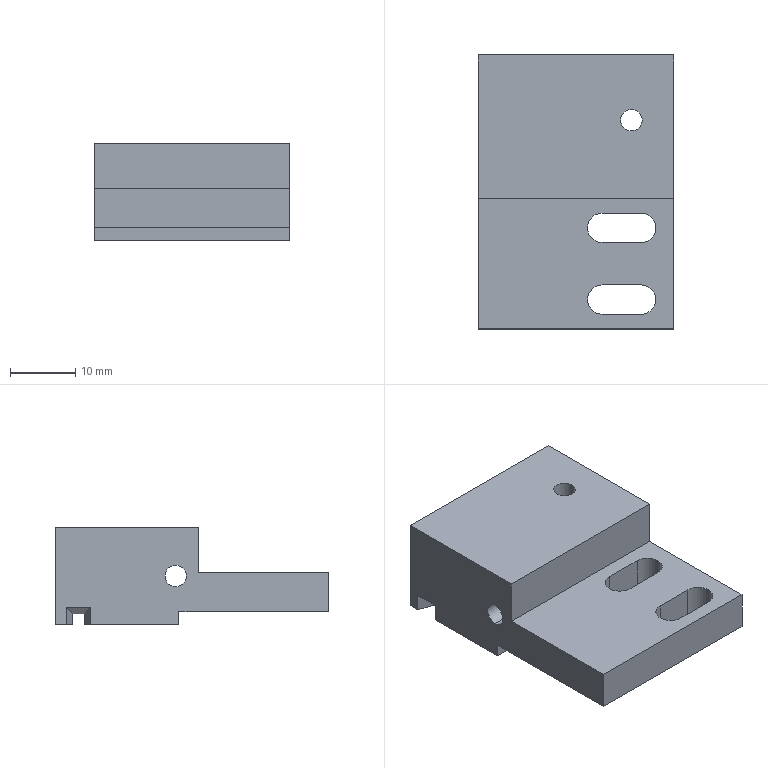Part | NX | features BREP 1 | 1 solid | 41 faces | box 30 x 42 x 15 mm | volume 11628 mm3 | plane 25 | cylinder 16 | commonest cylinder face diameters 4.5 x6 3.3 x4 10 x2 11.5 x2 14 x2
STEP:
#1=CARTESIAN_POINT('',(-23.5,-9.,-7.5));
#2=VERTEX_POINT('',#1);
#3=CARTESIAN_POINT('',(6.5,-9.,-7.5));
#4=VERTEX_POINT('',#3);
#5=CARTESIAN_POINT('',(6.5,-9.,-7.5));
#6=DIRECTION('',(1.,0.,0.));
#7=VECTOR('',#6,1000.);
#8=LINE('',#5,#7);
#9=EDGE_CURVE('',#2,#4,#8,.T.);
#10=ORIENTED_EDGE('',*,*,#9,.T.);
#11=CARTESIAN_POINT('',(6.5,-9.,-5.5));
#12=VERTEX_POINT('',#11);
#13=CARTESIAN_POINT('',(6.5,-9.,-5.5));
#14=DIRECTION('',(0.,0.,-1.));
#15=VECTOR('',#14,1000.);
#16=LINE('',#13,#15);
#17=EDGE_CURVE('',#12,#4,#16,.T.);
#18=ORIENTED_EDGE('',*,*,#17,.F.);
#19=CARTESIAN_POINT('',(-23.5,-9.,-5.5));
#20=VERTEX_POINT('',#19);
#21=CARTESIAN_POINT('',(6.5,-9.,-5.5));
#22=DIRECTION('',(1.,0.,0.));
#23=VECTOR('',#22,1000.);
#24=LINE('',#21,#23);
#25=EDGE_CURVE('',#20,#12,#24,.T.);
#26=ORIENTED_EDGE('',*,*,#25,.F.);
#27=CARTESIAN_POINT('',(-23.5,-9.,-5.5));
#28=DIRECTION('',(0.,0.,-1.));
#29=VECTOR('',#28,1000.);
#30=LINE('',#27,#29);
#31=EDGE_CURVE('',#20,#2,#30,.T.);
#32=ORIENTED_EDGE('',*,*,#31,.T.);
#33=EDGE_LOOP('',(#10,#18,#26,#32));
#34=FACE_BOUND('',#33,.T.);
#35=CARTESIAN_POINT('',(6.5,-9.,-5.5));
#36=DIRECTION('',(0.,1.,0.));
#37=DIRECTION('',(0.,0.,1.));
#38=AXIS2_PLACEMENT_3D('',#35,#36,#37);
#39=PLANE('',#38);
#40=ADVANCED_FACE('',(#34),#39,.F.);
#41=CARTESIAN_POINT('',(-4.5,-14.25,-5.5));
#42=VERTEX_POINT('',#41);
#43=CARTESIAN_POINT('',(-4.5,-18.75,-5.5));
#44=VERTEX_POINT('',#43);
#45=CARTESIAN_POINT('',(-4.5,-16.5,-5.5));
#46=DIRECTION('',(0.,0.,1.));
#47=DIRECTION('',(-1.,0.,0.));
#48=AXIS2_PLACEMENT_3D('',#45,#46,#47);
#49=CIRCLE('',#48,2.25);
#50=EDGE_CURVE('',#42,#44,#49,.T.);
#51=ORIENTED_EDGE('',*,*,#50,.T.);
#52=CARTESIAN_POINT('',(1.5,-18.75,-5.5));
#53=VERTEX_POINT('',#52);
#54=CARTESIAN_POINT('',(-4.5,-18.75,-5.5));
#55=DIRECTION('',(1.,0.,0.));
#56=VECTOR('',#55,1000.);
#57=LINE('',#54,#56);
#58=EDGE_CURVE('',#44,#53,#57,.T.);
#59=ORIENTED_EDGE('',*,*,#58,.T.);
#60=CARTESIAN_POINT('',(3.75,-16.5,-5.5));
#61=VERTEX_POINT('',#60);
#62=CARTESIAN_POINT('',(1.5,-16.5,-5.5));
#63=DIRECTION('',(0.,0.,1.));
#64=DIRECTION('',(-1.,0.,0.));
#65=AXIS2_PLACEMENT_3D('',#62,#63,#64);
#66=CIRCLE('',#65,2.25);
#67=EDGE_CURVE('',#53,#61,#66,.T.);
#68=ORIENTED_EDGE('',*,*,#67,.T.);
#69=CARTESIAN_POINT('',(1.5,-14.25,-5.5));
#70=VERTEX_POINT('',#69);
#71=CARTESIAN_POINT('',(1.5,-16.5,-5.5));
#72=DIRECTION('',(0.,0.,1.));
#73=DIRECTION('',(-1.,0.,0.));
#74=AXIS2_PLACEMENT_3D('',#71,#72,#73);
#75=CIRCLE('',#74,2.25);
#76=EDGE_CURVE('',#61,#70,#75,.T.);
#77=ORIENTED_EDGE('',*,*,#76,.T.);
#78=CARTESIAN_POINT('',(-4.5,-14.25,-5.5));
#79=DIRECTION('',(-1.,0.,0.));
#80=VECTOR('',#79,1000.);
#81=LINE('',#78,#80);
#82=EDGE_CURVE('',#70,#42,#81,.T.);
#83=ORIENTED_EDGE('',*,*,#82,.T.);
#84=EDGE_LOOP('',(#51,#59,#68,#77,#83));
#85=FACE_BOUND('',#84,.T.);
#86=CARTESIAN_POINT('',(-23.5,-32.,-5.5));
#87=VERTEX_POINT('',#86);
#88=CARTESIAN_POINT('',(-23.5,-9.,-5.5));
#89=DIRECTION('',(0.,1.,0.));
#90=VECTOR('',#89,1000.);
#91=LINE('',#88,#90);
#92=EDGE_CURVE('',#87,#20,#91,.T.);
#93=ORIENTED_EDGE('',*,*,#92,.T.);
#94=ORIENTED_EDGE('',*,*,#25,.T.);
#95=CARTESIAN_POINT('',(6.5,-32.,-5.5));
#96=VERTEX_POINT('',#95);
#97=CARTESIAN_POINT('',(6.5,-9.,-5.5));
#98=DIRECTION('',(0.,-1.,0.));
#99=VECTOR('',#98,1000.);
#100=LINE('',#97,#99);
#101=EDGE_CURVE('',#12,#96,#100,.T.);
#102=ORIENTED_EDGE('',*,*,#101,.T.);
#103=CARTESIAN_POINT('',(6.5,-32.,-5.5));
#104=DIRECTION('',(-1.,0.,0.));
#105=VECTOR('',#104,1000.);
#106=LINE('',#103,#105);
#107=EDGE_CURVE('',#96,#87,#106,.T.);
#108=ORIENTED_EDGE('',*,*,#107,.T.);
#109=EDGE_LOOP('',(#93,#94,#102,#108));
#110=FACE_BOUND('',#109,.T.);
#111=CARTESIAN_POINT('',(-4.5,-25.25,-5.5));
#112=VERTEX_POINT('',#111);
#113=CARTESIAN_POINT('',(-4.5,-29.75,-5.5));
#114=VERTEX_POINT('',#113);
#115=CARTESIAN_POINT('',(-4.5,-27.5,-5.5));
#116=DIRECTION('',(0.,0.,1.));
#117=DIRECTION('',(-1.,0.,0.));
#118=AXIS2_PLACEMENT_3D('',#115,#116,#117);
#119=CIRCLE('',#118,2.25);
#120=EDGE_CURVE('',#112,#114,#119,.T.);
#121=ORIENTED_EDGE('',*,*,#120,.T.);
#122=CARTESIAN_POINT('',(1.5,-29.75,-5.5));
#123=VERTEX_POINT('',#122);
#124=CARTESIAN_POINT('',(-4.5,-29.75,-5.5));
#125=DIRECTION('',(1.,0.,0.));
#126=VECTOR('',#125,1000.);
#127=LINE('',#124,#126);
#128=EDGE_CURVE('',#114,#123,#127,.T.);
#129=ORIENTED_EDGE('',*,*,#128,.T.);
#130=CARTESIAN_POINT('',(3.75,-27.5,-5.5));
#131=VERTEX_POINT('',#130);
#132=CARTESIAN_POINT('',(1.5,-27.5,-5.5));
#133=DIRECTION('',(0.,0.,1.));
#134=DIRECTION('',(-1.,0.,0.));
#135=AXIS2_PLACEMENT_3D('',#132,#133,#134);
#136=CIRCLE('',#135,2.25);
#137=EDGE_CURVE('',#123,#131,#136,.T.);
#138=ORIENTED_EDGE('',*,*,#137,.T.);
#139=CARTESIAN_POINT('',(1.5,-25.25,-5.5));
#140=VERTEX_POINT('',#139);
#141=CARTESIAN_POINT('',(1.5,-27.5,-5.5));
#142=DIRECTION('',(0.,0.,1.));
#143=DIRECTION('',(-1.,0.,0.));
#144=AXIS2_PLACEMENT_3D('',#141,#142,#143);
#145=CIRCLE('',#144,2.25);
#146=EDGE_CURVE('',#131,#140,#145,.T.);
#147=ORIENTED_EDGE('',*,*,#146,.T.);
#148=CARTESIAN_POINT('',(-4.5,-25.25,-5.5));
#149=DIRECTION('',(-1.,0.,0.));
#150=VECTOR('',#149,1000.);
#151=LINE('',#148,#150);
#152=EDGE_CURVE('',#140,#112,#151,.T.);
#153=ORIENTED_EDGE('',*,*,#152,.T.);
#154=EDGE_LOOP('',(#121,#129,#138,#147,#153));
#155=FACE_BOUND('',#154,.T.);
#156=CARTESIAN_POINT('',(0.,0.,-5.5));
#157=DIRECTION('',(0.,0.,-1.));
#158=DIRECTION('',(-1.,0.,0.));
#159=AXIS2_PLACEMENT_3D('',#156,#157,#158);
#160=PLANE('',#159);
#161=ADVANCED_FACE('',(#85,#110,#155),#160,.T.);
#162=CARTESIAN_POINT('',(-5.75,0.,-4.3));
#163=VERTEX_POINT('',#162);
#164=CARTESIAN_POINT('',(5.75,0.,-4.3));
#165=VERTEX_POINT('',#164);
#166=CARTESIAN_POINT('',(0.,0.,-4.3));
#167=DIRECTION('',(0.,0.,-1.));
#168=DIRECTION('',(-1.,0.,0.));
#169=AXIS2_PLACEMENT_3D('',#166,#167,#168);
#170=CIRCLE('',#169,5.75);
#171=EDGE_CURVE('',#163,#165,#170,.T.);
#172=ORIENTED_EDGE('',*,*,#171,.T.);
#173=CARTESIAN_POINT('',(0.,0.,-4.3));
#174=DIRECTION('',(0.,0.,-1.));
#175=DIRECTION('',(-1.,0.,0.));
#176=AXIS2_PLACEMENT_3D('',#173,#174,#175);
#177=CIRCLE('',#176,5.75);
#178=EDGE_CURVE('',#165,#163,#177,.T.);
#179=ORIENTED_EDGE('',*,*,#178,.T.);
#180=EDGE_LOOP('',(#172,#179));
#181=FACE_BOUND('',#180,.T.);
#182=CARTESIAN_POINT('',(-5.,0.,-4.3));
#183=VERTEX_POINT('',#182);
#184=CARTESIAN_POINT('',(5.,0.,-4.3));
#185=VERTEX_POINT('',#184);
#186=CARTESIAN_POINT('',(0.,0.,-4.3));
#187=DIRECTION('',(0.,0.,-1.));
#188=DIRECTION('',(-1.,0.,0.));
#189=AXIS2_PLACEMENT_3D('',#186,#187,#188);
#190=CIRCLE('',#189,5.);
#191=EDGE_CURVE('',#183,#185,#190,.T.);
#192=ORIENTED_EDGE('',*,*,#191,.F.);
#193=CARTESIAN_POINT('',(0.,0.,-4.3));
#194=DIRECTION('',(0.,0.,-1.));
#195=DIRECTION('',(-1.,0.,0.));
#196=AXIS2_PLACEMENT_3D('',#193,#194,#195);
#197=CIRCLE('',#196,5.);
#198=EDGE_CURVE('',#185,#183,#197,.T.);
#199=ORIENTED_EDGE('',*,*,#198,.F.);
#200=EDGE_LOOP('',(#192,#199));
#201=FACE_BOUND('',#200,.T.);
#202=CARTESIAN_POINT('',(0.,0.,-4.3));
#203=DIRECTION('',(0.,0.,-1.));
#204=DIRECTION('',(-1.,0.,0.));
#205=AXIS2_PLACEMENT_3D('',#202,#203,#204);
#206=PLANE('',#205);
#207=ADVANCED_FACE('',(#181,#201),#206,.T.);
#208=CARTESIAN_POINT('',(5.75,0.,-5.8));
#209=VERTEX_POINT('',#208);
#210=CARTESIAN_POINT('',(5.75,0.,-4.3));
#211=DIRECTION('',(0.,0.,-1.));
#212=VECTOR('',#211,1000.);
#213=LINE('',#210,#212);
#214=EDGE_CURVE('',#165,#209,#213,.T.);
#215=ORIENTED_EDGE('',*,*,#214,.F.);
#216=ORIENTED_EDGE('',*,*,#171,.F.);
#217=CARTESIAN_POINT('',(-5.75,0.,-5.8));
#218=VERTEX_POINT('',#217);
#219=CARTESIAN_POINT('',(-5.75,0.,-4.3));
#220=DIRECTION('',(0.,0.,-1.));
#221=VECTOR('',#220,1000.);
#222=LINE('',#219,#221);
#223=EDGE_CURVE('',#163,#218,#222,.T.);
#224=ORIENTED_EDGE('',*,*,#223,.T.);
#225=CARTESIAN_POINT('',(0.,0.,-5.8));
#226=DIRECTION('',(0.,0.,-1.));
#227=DIRECTION('',(-1.,0.,0.));
#228=AXIS2_PLACEMENT_3D('',#225,#226,#227);
#229=CIRCLE('',#228,5.75);
#230=EDGE_CURVE('',#218,#209,#229,.T.);
#231=ORIENTED_EDGE('',*,*,#230,.T.);
#232=EDGE_LOOP('',(#215,#216,#224,#231));
#233=FACE_BOUND('',#232,.T.);
#234=CARTESIAN_POINT('',(0.,0.,-4.3));
#235=DIRECTION('',(0.,0.,-1.));
#236=DIRECTION('',(-1.,0.,0.));
#237=AXIS2_PLACEMENT_3D('',#234,#235,#236);
#238=CYLINDRICAL_SURFACE('',#237,5.75);
#239=ADVANCED_FACE('',(#233),#238,.F.);
#240=CARTESIAN_POINT('',(-23.5,-8.5,-1.65));
#241=VERTEX_POINT('',#240);
#242=CARTESIAN_POINT('',(6.5,-8.5,-1.65));
#243=VERTEX_POINT('',#242);
#244=CARTESIAN_POINT('',(-23.5,-8.5,-1.65));
#245=DIRECTION('',(-1.,0.,0.));
#246=VECTOR('',#245,1000.);
#247=LINE('',#244,#246);
#248=EDGE_CURVE('',#241,#243,#247,.F.);
#249=ORIENTED_EDGE('',*,*,#248,.T.);
#250=CARTESIAN_POINT('',(6.5,-8.5,1.65));
#251=VERTEX_POINT('',#250);
#252=CARTESIAN_POINT('',(6.5,-8.5,0.));
#253=DIRECTION('',(-1.,0.,0.));
#254=DIRECTION('',(0.,0.,1.));
#255=AXIS2_PLACEMENT_3D('',#252,#253,#254);
#256=CIRCLE('',#255,1.65);
#257=EDGE_CURVE('',#251,#243,#256,.T.);
#258=ORIENTED_EDGE('',*,*,#257,.F.);
#259=CARTESIAN_POINT('',(-23.5,-8.5,1.65));
#260=VERTEX_POINT('',#259);
#261=CARTESIAN_POINT('',(-23.5,-8.5,1.65));
#262=DIRECTION('',(-1.,0.,0.));
#263=VECTOR('',#262,1000.);
#264=LINE('',#261,#263);
#265=EDGE_CURVE('',#260,#251,#264,.F.);
#266=ORIENTED_EDGE('',*,*,#265,.F.);
#267=CARTESIAN_POINT('',(-23.5,-8.5,0.));
#268=DIRECTION('',(-1.,0.,0.));
#269=DIRECTION('',(0.,0.,1.));
#270=AXIS2_PLACEMENT_3D('',#267,#268,#269);
#271=CIRCLE('',#270,1.65);
#272=EDGE_CURVE('',#260,#241,#271,.T.);
#273=ORIENTED_EDGE('',*,*,#272,.T.);
#274=EDGE_LOOP('',(#249,#258,#266,#273));
#275=FACE_BOUND('',#274,.T.);
#276=CARTESIAN_POINT('',(-23.5,-8.5,0.));
#277=DIRECTION('',(-1.,0.,0.));
#278=DIRECTION('',(0.,0.,1.));
#279=AXIS2_PLACEMENT_3D('',#276,#277,#278);
#280=CYLINDRICAL_SURFACE('',#279,1.65);
#281=ADVANCED_FACE('',(#275),#280,.F.);
#282=CARTESIAN_POINT('',(-4.899,5.5,-5.8));
#283=VERTEX_POINT('',#282);
#284=CARTESIAN_POINT('',(-4.899,5.,-5.8));
#285=VERTEX_POINT('',#284);
#286=CARTESIAN_POINT('',(-4.899,5.5,-5.8));
#287=DIRECTION('',(0.,-1.,0.));
#288=VECTOR('',#287,1000.);
#289=LINE('',#286,#288);
#290=EDGE_CURVE('',#283,#285,#289,.T.);
#291=ORIENTED_EDGE('',*,*,#290,.T.);
#292=CARTESIAN_POINT('',(-4.899,5.,-7.5));
#293=VERTEX_POINT('',#292);
#294=CARTESIAN_POINT('',(-4.899,5.,-5.043));
#295=DIRECTION('',(0.,0.,-1.));
#296=VECTOR('',#295,1000.);
#297=LINE('',#294,#296);
#298=EDGE_CURVE('',#285,#293,#297,.T.);
#299=ORIENTED_EDGE('',*,*,#298,.T.);
#300=CARTESIAN_POINT('',(-4.899,5.5,-7.5));
#301=VERTEX_POINT('',#300);
#302=CARTESIAN_POINT('',(-4.899,5.5,-7.5));
#303=DIRECTION('',(0.,-1.,0.));
#304=VECTOR('',#303,1000.);
#305=LINE('',#302,#304);
#306=EDGE_CURVE('',#301,#293,#305,.T.);
#307=ORIENTED_EDGE('',*,*,#306,.F.);
#308=CARTESIAN_POINT('',(-4.899,5.5,-5.043));
#309=DIRECTION('',(0.,0.,-1.));
#310=VECTOR('',#309,1000.);
#311=LINE('',#308,#310);
#312=EDGE_CURVE('',#283,#301,#311,.T.);
#313=ORIENTED_EDGE('',*,*,#312,.F.);
#314=EDGE_LOOP('',(#291,#299,#307,#313));
#315=FACE_BOUND('',#314,.T.);
#316=CARTESIAN_POINT('',(-4.899,5.5,-5.043));
#317=DIRECTION('',(1.,0.,0.));
#318=DIRECTION('',(0.,0.,-1.));
#319=AXIS2_PLACEMENT_3D('',#316,#317,#318);
#320=PLANE('',#319);
#321=ADVANCED_FACE('',(#315),#320,.T.);
#322=CARTESIAN_POINT('',(-23.5,4.5,-4.8));
#323=VERTEX_POINT('',#322);
#324=CARTESIAN_POINT('',(-20.5,5.5,-5.8));
#325=VERTEX_POINT('',#324);
#326=CARTESIAN_POINT('',(-26.855,3.382,-3.682));
#327=DIRECTION('',(0.9045,0.3015,-0.3015));
#328=VECTOR('',#327,1000.);
#329=LINE('',#326,#328);
#330=EDGE_CURVE('',#323,#325,#329,.T.);
#331=ORIENTED_EDGE('',*,*,#330,.T.);
#332=CARTESIAN_POINT('',(-20.5,5.5,-7.5));
#333=VERTEX_POINT('',#332);
#334=CARTESIAN_POINT('',(-20.5,5.5,-5.8));
#335=DIRECTION('',(0.,0.,1.));
#336=VECTOR('',#335,1000.);
#337=LINE('',#334,#336);
#338=EDGE_CURVE('',#333,#325,#337,.T.);
#339=ORIENTED_EDGE('',*,*,#338,.F.);
#340=CARTESIAN_POINT('',(-23.5,4.5,-7.5));
#341=VERTEX_POINT('',#340);
#342=CARTESIAN_POINT('',(-3.7,11.1,-7.5));
#343=DIRECTION('',(0.9487,0.3162,0.));
#344=VECTOR('',#343,1000.);
#345=LINE('',#342,#344);
#346=EDGE_CURVE('',#341,#333,#345,.T.);
#347=ORIENTED_EDGE('',*,*,#346,.F.);
#348=CARTESIAN_POINT('',(-23.5,4.5,-7.5));
#349=DIRECTION('',(0.,0.,-1.));
#350=VECTOR('',#349,1000.);
#351=LINE('',#348,#350);
#352=EDGE_CURVE('',#323,#341,#351,.T.);
#353=ORIENTED_EDGE('',*,*,#352,.F.);
#354=EDGE_LOOP('',(#331,#339,#347,#353));
#355=FACE_BOUND('',#354,.T.);
#356=CARTESIAN_POINT('',(-23.5,4.5,7.5));
#357=DIRECTION('',(-0.3162,0.9487,0.));
#358=DIRECTION('',(0.,0.,1.));
#359=AXIS2_PLACEMENT_3D('',#356,#357,#358);
#360=PLANE('',#359);
#361=ADVANCED_FACE('',(#355),#360,.T.);
#362=CARTESIAN_POINT('',(-23.5,8.3,-4.8));
#363=VERTEX_POINT('',#362);
#364=CARTESIAN_POINT('',(-20.5,7.3,-5.8));
#365=VERTEX_POINT('',#364);
#366=CARTESIAN_POINT('',(-12.509,4.636,-8.464));
#367=DIRECTION('',(0.9045,-0.3015,-0.3015));
#368=VECTOR('',#367,1000.);
#369=LINE('',#366,#368);
#370=EDGE_CURVE('',#363,#365,#369,.T.);
#371=ORIENTED_EDGE('',*,*,#370,.T.);
#372=CARTESIAN_POINT('',(-20.5,0.,-5.8));
#373=DIRECTION('',(0.,1.,0.));
#374=VECTOR('',#373,1000.);
#375=LINE('',#372,#374);
#376=EDGE_CURVE('',#325,#365,#375,.T.);
#377=ORIENTED_EDGE('',*,*,#376,.F.);
#378=ORIENTED_EDGE('',*,*,#330,.F.);
#379=CARTESIAN_POINT('',(-23.5,-32.,-4.8));
#380=DIRECTION('',(0.,-1.,0.));
#381=VECTOR('',#380,1000.);
#382=LINE('',#379,#381);
#383=EDGE_CURVE('',#363,#323,#382,.T.);
#384=ORIENTED_EDGE('',*,*,#383,.F.);
#385=EDGE_LOOP('',(#371,#377,#378,#384));
#386=FACE_BOUND('',#385,.T.);
#387=CARTESIAN_POINT('',(-23.5,-32.,-4.8));
#388=DIRECTION('',(0.3162,0.,0.9487));
#389=DIRECTION('',(0.,-1.,0.));
#390=AXIS2_PLACEMENT_3D('',#387,#388,#389);
#391=PLANE('',#390);
#392=ADVANCED_FACE('',(#386),#391,.F.);
#393=CARTESIAN_POINT('',(-20.5,7.3,-7.5));
#394=VERTEX_POINT('',#393);
#395=CARTESIAN_POINT('',(-23.5,8.3,-7.5));
#396=VERTEX_POINT('',#395);
#397=CARTESIAN_POINT('',(0.14,0.42,-7.5));
#398=DIRECTION('',(-0.9487,0.3162,0.));
#399=VECTOR('',#398,1000.);
#400=LINE('',#397,#399);
#401=EDGE_CURVE('',#394,#396,#400,.T.);
#402=ORIENTED_EDGE('',*,*,#401,.F.);
#403=CARTESIAN_POINT('',(-20.5,7.3,-7.5));
#404=DIRECTION('',(0.,0.,-1.));
#405=VECTOR('',#404,1000.);
#406=LINE('',#403,#405);
#407=EDGE_CURVE('',#365,#394,#406,.T.);
#408=ORIENTED_EDGE('',*,*,#407,.F.);
#409=ORIENTED_EDGE('',*,*,#370,.F.);
#410=CARTESIAN_POINT('',(-23.5,8.3,-5.8));
#411=DIRECTION('',(0.,0.,1.));
#412=VECTOR('',#411,1000.);
#413=LINE('',#410,#412);
#414=EDGE_CURVE('',#396,#363,#413,.T.);
#415=ORIENTED_EDGE('',*,*,#414,.F.);
#416=EDGE_LOOP('',(#402,#408,#409,#415));
#417=FACE_BOUND('',#416,.T.);
#418=CARTESIAN_POINT('',(-20.5,7.3,-5.8));
#419=DIRECTION('',(-0.3162,-0.9487,0.));
#420=DIRECTION('',(0.,0.,1.));
#421=AXIS2_PLACEMENT_3D('',#418,#419,#420);
#422=PLANE('',#421);
#423=ADVANCED_FACE('',(#417),#422,.T.);
#424=CARTESIAN_POINT('',(6.5,-7.,-5.8));
#425=VERTEX_POINT('',#424);
#426=CARTESIAN_POINT('',(6.5,-7.,-7.5));
#427=VERTEX_POINT('',#426);
#428=CARTESIAN_POINT('',(6.5,-7.,7.5));
#429=DIRECTION('',(0.,0.,-1.));
#430=VECTOR('',#429,1000.);
#431=LINE('',#428,#430);
#432=EDGE_CURVE('',#425,#427,#431,.T.);
#433=ORIENTED_EDGE('',*,*,#432,.T.);
#434=CARTESIAN_POINT('',(0.,-7.,-7.5));
#435=VERTEX_POINT('',#434);
#436=CARTESIAN_POINT('',(0.,-7.,-7.5));
#437=DIRECTION('',(1.,0.,0.));
#438=VECTOR('',#437,1000.);
#439=LINE('',#436,#438);
#440=EDGE_CURVE('',#435,#427,#439,.T.);
#441=ORIENTED_EDGE('',*,*,#440,.F.);
#442=CARTESIAN_POINT('',(0.,-7.,-5.8));
#443=VERTEX_POINT('',#442);
#444=CARTESIAN_POINT('',(0.,-7.,17.743));
#445=DIRECTION('',(0.,0.,-1.));
#446=VECTOR('',#445,1000.);
#447=LINE('',#444,#446);
#448=EDGE_CURVE('',#443,#435,#447,.T.);
#449=ORIENTED_EDGE('',*,*,#448,.F.);
#450=CARTESIAN_POINT('',(0.,-7.,-5.8));
#451=DIRECTION('',(1.,0.,0.));
#452=VECTOR('',#451,1000.);
#453=LINE('',#450,#452);
#454=EDGE_CURVE('',#443,#425,#453,.T.);
#455=ORIENTED_EDGE('',*,*,#454,.T.);
#456=EDGE_LOOP('',(#433,#441,#449,#455));
#457=FACE_BOUND('',#456,.T.);
#458=CARTESIAN_POINT('',(0.,-7.,17.743));
#459=DIRECTION('',(0.,1.,0.));
#460=DIRECTION('',(0.,0.,1.));
#461=AXIS2_PLACEMENT_3D('',#458,#459,#460);
#462=PLANE('',#461);
#463=ADVANCED_FACE('',(#457),#462,.T.);
#464=ORIENTED_EDGE('',*,*,#290,.F.);
#465=CARTESIAN_POINT('',(-23.5,5.5,-5.8));
#466=DIRECTION('',(1.,0.,0.));
#467=VECTOR('',#466,1000.);
#468=LINE('',#465,#467);
#469=EDGE_CURVE('',#325,#283,#468,.T.);
#470=ORIENTED_EDGE('',*,*,#469,.F.);
#471=ORIENTED_EDGE('',*,*,#376,.T.);
#472=CARTESIAN_POINT('',(6.5,7.3,-5.8));
#473=VERTEX_POINT('',#472);
#474=CARTESIAN_POINT('',(-23.5,7.3,-5.8));
#475=DIRECTION('',(-1.,0.,0.));
#476=VECTOR('',#475,1000.);
#477=LINE('',#474,#476);
#478=EDGE_CURVE('',#473,#365,#477,.T.);
#479=ORIENTED_EDGE('',*,*,#478,.F.);
#480=CARTESIAN_POINT('',(6.5,7.3,-5.8));
#481=DIRECTION('',(0.,1.,0.));
#482=VECTOR('',#481,1000.);
#483=LINE('',#480,#482);
#484=EDGE_CURVE('',#425,#473,#483,.T.);
#485=ORIENTED_EDGE('',*,*,#484,.F.);
#486=ORIENTED_EDGE('',*,*,#454,.F.);
#487=CARTESIAN_POINT('',(-7.,0.,-5.8));
#488=VERTEX_POINT('',#487);
#489=CARTESIAN_POINT('',(0.,0.,-5.8));
#490=DIRECTION('',(0.,0.,1.));
#491=DIRECTION('',(1.,0.,0.));
#492=AXIS2_PLACEMENT_3D('',#489,#490,#491);
#493=CIRCLE('',#492,7.);
#494=EDGE_CURVE('',#488,#443,#493,.T.);
#495=ORIENTED_EDGE('',*,*,#494,.F.);
#496=CARTESIAN_POINT('',(0.,0.,-5.8));
#497=DIRECTION('',(0.,0.,1.));
#498=DIRECTION('',(1.,0.,0.));
#499=AXIS2_PLACEMENT_3D('',#496,#497,#498);
#500=CIRCLE('',#499,7.);
#501=EDGE_CURVE('',#285,#488,#500,.T.);
#502=ORIENTED_EDGE('',*,*,#501,.F.);
#503=EDGE_LOOP('',(#464,#470,#471,#479,#485,#486,#495,#502));
#504=FACE_BOUND('',#503,.T.);
#505=ORIENTED_EDGE('',*,*,#230,.F.);
#506=CARTESIAN_POINT('',(0.,0.,-5.8));
#507=DIRECTION('',(0.,0.,-1.));
#508=DIRECTION('',(-1.,0.,0.));
#509=AXIS2_PLACEMENT_3D('',#506,#507,#508);
#510=CIRCLE('',#509,5.75);
#511=EDGE_CURVE('',#209,#218,#510,.T.);
#512=ORIENTED_EDGE('',*,*,#511,.F.);
#513=EDGE_LOOP('',(#505,#512));
#514=FACE_BOUND('',#513,.T.);
#515=CARTESIAN_POINT('',(0.,0.,-5.8));
#516=DIRECTION('',(0.,0.,1.));
#517=DIRECTION('',(1.,0.,0.));
#518=AXIS2_PLACEMENT_3D('',#515,#516,#517);
#519=PLANE('',#518);
#520=ADVANCED_FACE('',(#504,#514),#519,.F.);
#521=ORIENTED_EDGE('',*,*,#478,.T.);
#522=ORIENTED_EDGE('',*,*,#407,.T.);
#523=CARTESIAN_POINT('',(6.5,7.3,-7.5));
#524=VERTEX_POINT('',#523);
#525=CARTESIAN_POINT('',(-23.5,7.3,-7.5));
#526=DIRECTION('',(-1.,0.,0.));
#527=VECTOR('',#526,1000.);
#528=LINE('',#525,#527);
#529=EDGE_CURVE('',#524,#394,#528,.T.);
#530=ORIENTED_EDGE('',*,*,#529,.F.);
#531=CARTESIAN_POINT('',(6.5,7.3,-5.8));
#532=DIRECTION('',(0.,0.,-1.));
#533=VECTOR('',#532,1000.);
#534=LINE('',#531,#533);
#535=EDGE_CURVE('',#473,#524,#534,.T.);
#536=ORIENTED_EDGE('',*,*,#535,.F.);
#537=EDGE_LOOP('',(#521,#522,#530,#536));
#538=FACE_BOUND('',#537,.T.);
#539=CARTESIAN_POINT('',(-23.5,7.3,-5.8));
#540=DIRECTION('',(0.,-1.,0.));
#541=DIRECTION('',(0.,0.,-1.));
#542=AXIS2_PLACEMENT_3D('',#539,#540,#541);
#543=PLANE('',#542);
#544=ADVANCED_FACE('',(#538),#543,.T.);
#545=CARTESIAN_POINT('',(1.65,0.,7.5));
#546=VERTEX_POINT('',#545);
#547=CARTESIAN_POINT('',(1.65,0.,0.));
#548=VERTEX_POINT('',#547);
#549=CARTESIAN_POINT('',(1.65,0.,0.));
#550=DIRECTION('',(0.,0.,-1.));
#551=VECTOR('',#550,1000.);
#552=LINE('',#549,#551);
#553=EDGE_CURVE('',#546,#548,#552,.T.);
#554=ORIENTED_EDGE('',*,*,#553,.F.);
#555=CARTESIAN_POINT('',(-1.65,0.,7.5));
#556=VERTEX_POINT('',#555);
#557=CARTESIAN_POINT('',(0.,0.,7.5));
#558=DIRECTION('',(0.,0.,-1.));
#559=DIRECTION('',(-1.,0.,0.));
#560=AXIS2_PLACEMENT_3D('',#557,#558,#559);
#561=CIRCLE('',#560,1.65);
#562=EDGE_CURVE('',#556,#546,#561,.T.);
#563=ORIENTED_EDGE('',*,*,#562,.F.);
#564=CARTESIAN_POINT('',(-1.65,0.,0.));
#565=VERTEX_POINT('',#564);
#566=CARTESIAN_POINT('',(-1.65,0.,0.));
#567=DIRECTION('',(0.,0.,-1.));
#568=VECTOR('',#567,1000.);
#569=LINE('',#566,#568);
#570=EDGE_CURVE('',#556,#565,#569,.T.);
#571=ORIENTED_EDGE('',*,*,#570,.T.);
#572=CARTESIAN_POINT('',(0.,0.,0.));
#573=DIRECTION('',(0.,0.,-1.));
#574=DIRECTION('',(-1.,0.,0.));
#575=AXIS2_PLACEMENT_3D('',#572,#573,#574);
#576=CIRCLE('',#575,1.65);
#577=EDGE_CURVE('',#565,#548,#576,.T.);
#578=ORIENTED_EDGE('',*,*,#577,.T.);
#579=EDGE_LOOP('',(#554,#563,#571,#578));
#580=FACE_BOUND('',#579,.T.);
#581=CARTESIAN_POINT('',(0.,0.,0.));
#582=DIRECTION('',(0.,0.,-1.));
#583=DIRECTION('',(-1.,0.,0.));
#584=AXIS2_PLACEMENT_3D('',#581,#582,#583);
#585=CYLINDRICAL_SURFACE('',#584,1.65);
#586=ADVANCED_FACE('',(#580),#585,.F.);
#587=CARTESIAN_POINT('',(-5.,0.,0.));
#588=VERTEX_POINT('',#587);
#589=CARTESIAN_POINT('',(5.,0.,0.));
#590=VERTEX_POINT('',#589);
#591=CARTESIAN_POINT('',(0.,0.,0.));
#592=DIRECTION('',(0.,0.,-1.));
#593=DIRECTION('',(-1.,0.,0.));
#594=AXIS2_PLACEMENT_3D('',#591,#592,#593);
#595=CIRCLE('',#594,5.);
#596=EDGE_CURVE('',#588,#590,#595,.T.);
#597=ORIENTED_EDGE('',*,*,#596,.T.);
#598=CARTESIAN_POINT('',(0.,0.,0.));
#599=DIRECTION('',(0.,0.,-1.));
#600=DIRECTION('',(-1.,0.,0.));
#601=AXIS2_PLACEMENT_3D('',#598,#599,#600);
#602=CIRCLE('',#601,5.);
#603=EDGE_CURVE('',#590,#588,#602,.T.);
#604=ORIENTED_EDGE('',*,*,#603,.T.);
#605=EDGE_LOOP('',(#597,#604));
#606=FACE_BOUND('',#605,.T.);
#607=ORIENTED_EDGE('',*,*,#577,.F.);
#608=CARTESIAN_POINT('',(0.,0.,0.));
#609=DIRECTION('',(0.,0.,-1.));
#610=DIRECTION('',(-1.,0.,0.));
#611=AXIS2_PLACEMENT_3D('',#608,#609,#610);
#612=CIRCLE('',#611,1.65);
#613=EDGE_CURVE('',#548,#565,#612,.T.);
#614=ORIENTED_EDGE('',*,*,#613,.F.);
#615=EDGE_LOOP('',(#607,#614));
#616=FACE_BOUND('',#615,.T.);
#617=CARTESIAN_POINT('',(0.,0.,0.));
#618=DIRECTION('',(0.,0.,-1.));
#619=DIRECTION('',(-1.,0.,0.));
#620=AXIS2_PLACEMENT_3D('',#617,#618,#619);
#621=PLANE('',#620);
#622=ADVANCED_FACE('',(#606,#616),#621,.T.);
#623=CARTESIAN_POINT('',(6.5,-12.,7.5));
#624=VERTEX_POINT('',#623);
#625=CARTESIAN_POINT('',(-23.5,-12.,7.5));
#626=VERTEX_POINT('',#625);
#627=CARTESIAN_POINT('',(9.5,-12.,7.5));
#628=DIRECTION('',(-1.,0.,0.));
#629=VECTOR('',#628,1000.);
#630=LINE('',#627,#629);
#631=EDGE_CURVE('',#624,#626,#630,.T.);
#632=ORIENTED_EDGE('',*,*,#631,.T.);
#633=CARTESIAN_POINT('',(-23.5,-12.,0.5));
#634=VERTEX_POINT('',#633);
#635=CARTESIAN_POINT('',(-23.5,-12.,0.5));
#636=DIRECTION('',(0.,0.,-1.));
#637=VECTOR('',#636,1000.);
#638=LINE('',#635,#637);
#639=EDGE_CURVE('',#626,#634,#638,.T.);
#640=ORIENTED_EDGE('',*,*,#639,.T.);
#641=CARTESIAN_POINT('',(6.5,-12.,0.5));
#642=VERTEX_POINT('',#641);
#643=CARTESIAN_POINT('',(9.5,-12.,0.5));
#644=DIRECTION('',(-1.,0.,0.));
#645=VECTOR('',#644,1000.);
#646=LINE('',#643,#645);
#647=EDGE_CURVE('',#642,#634,#646,.T.);
#648=ORIENTED_EDGE('',*,*,#647,.F.);
#649=CARTESIAN_POINT('',(6.5,-12.,7.5));
#650=DIRECTION('',(0.,0.,-1.));
#651=VECTOR('',#650,1000.);
#652=LINE('',#649,#651);
#653=EDGE_CURVE('',#624,#642,#652,.T.);
#654=ORIENTED_EDGE('',*,*,#653,.F.);
#655=EDGE_LOOP('',(#632,#640,#648,#654));
#656=FACE_BOUND('',#655,.T.);
#657=CARTESIAN_POINT('',(9.5,-12.,0.5));
#658=DIRECTION('',(0.,1.,0.));
#659=DIRECTION('',(0.,0.,1.));
#660=AXIS2_PLACEMENT_3D('',#657,#658,#659);
#661=PLANE('',#660);
#662=ADVANCED_FACE('',(#656),#661,.F.);
#663=ORIENTED_EDGE('',*,*,#647,.T.);
#664=CARTESIAN_POINT('',(-23.5,-32.,0.5));
#665=VERTEX_POINT('',#664);
#666=CARTESIAN_POINT('',(-23.5,-32.,0.5));
#667=DIRECTION('',(0.,-1.,0.));
#668=VECTOR('',#667,1000.);
#669=LINE('',#666,#668);
#670=EDGE_CURVE('',#634,#665,#669,.T.);
#671=ORIENTED_EDGE('',*,*,#670,.T.);
#672=CARTESIAN_POINT('',(6.5,-32.,0.5));
#673=VERTEX_POINT('',#672);
#674=CARTESIAN_POINT('',(9.5,-32.,0.5));
#675=DIRECTION('',(-1.,0.,0.));
#676=VECTOR('',#675,1000.);
#677=LINE('',#674,#676);
#678=EDGE_CURVE('',#673,#665,#677,.T.);
#679=ORIENTED_EDGE('',*,*,#678,.F.);
#680=CARTESIAN_POINT('',(6.5,10.,0.5));
#681=DIRECTION('',(0.,-1.,0.));
#682=VECTOR('',#681,1000.);
#683=LINE('',#680,#682);
#684=EDGE_CURVE('',#642,#673,#683,.T.);
#685=ORIENTED_EDGE('',*,*,#684,.F.);
#686=EDGE_LOOP('',(#663,#671,#679,#685));
#687=FACE_BOUND('',#686,.T.);
#688=CARTESIAN_POINT('',(1.5,-18.75,0.5));
#689=VERTEX_POINT('',#688);
#690=CARTESIAN_POINT('',(-4.5,-18.75,0.5));
#691=VERTEX_POINT('',#690);
#692=CARTESIAN_POINT('',(9.5,-18.75,0.5));
#693=DIRECTION('',(-1.,0.,0.));
#694=VECTOR('',#693,1000.);
#695=LINE('',#692,#694);
#696=EDGE_CURVE('',#689,#691,#695,.T.);
#697=ORIENTED_EDGE('',*,*,#696,.T.);
#698=CARTESIAN_POINT('',(-4.5,-14.25,0.5));
#699=VERTEX_POINT('',#698);
#700=CARTESIAN_POINT('',(-4.5,-16.5,0.5));
#701=DIRECTION('',(0.,0.,-1.));
#702=DIRECTION('',(-1.,0.,0.));
#703=AXIS2_PLACEMENT_3D('',#700,#701,#702);
#704=CIRCLE('',#703,2.25);
#705=EDGE_CURVE('',#691,#699,#704,.T.);
#706=ORIENTED_EDGE('',*,*,#705,.T.);
#707=CARTESIAN_POINT('',(1.5,-14.25,0.5));
#708=VERTEX_POINT('',#707);
#709=CARTESIAN_POINT('',(9.5,-14.25,0.5));
#710=DIRECTION('',(1.,0.,0.));
#711=VECTOR('',#710,1000.);
#712=LINE('',#709,#711);
#713=EDGE_CURVE('',#699,#708,#712,.T.);
#714=ORIENTED_EDGE('',*,*,#713,.T.);
#715=CARTESIAN_POINT('',(3.75,-16.5,0.5));
#716=VERTEX_POINT('',#715);
#717=CARTESIAN_POINT('',(1.5,-16.5,0.5));
#718=DIRECTION('',(0.,0.,-1.));
#719=DIRECTION('',(-1.,0.,0.));
#720=AXIS2_PLACEMENT_3D('',#717,#718,#719);
#721=CIRCLE('',#720,2.25);
#722=EDGE_CURVE('',#708,#716,#721,.T.);
#723=ORIENTED_EDGE('',*,*,#722,.T.);
#724=CARTESIAN_POINT('',(1.5,-16.5,0.5));
#725=DIRECTION('',(0.,0.,-1.));
#726=DIRECTION('',(-1.,0.,0.));
#727=AXIS2_PLACEMENT_3D('',#724,#725,#726);
#728=CIRCLE('',#727,2.25);
#729=EDGE_CURVE('',#716,#689,#728,.T.);
#730=ORIENTED_EDGE('',*,*,#729,.T.);
#731=EDGE_LOOP('',(#697,#706,#714,#723,#730));
#732=FACE_BOUND('',#731,.T.);
#733=CARTESIAN_POINT('',(1.5,-29.75,0.5));
#734=VERTEX_POINT('',#733);
#735=CARTESIAN_POINT('',(-4.5,-29.75,0.5));
#736=VERTEX_POINT('',#735);
#737=CARTESIAN_POINT('',(9.5,-29.75,0.5));
#738=DIRECTION('',(-1.,0.,0.));
#739=VECTOR('',#738,1000.);
#740=LINE('',#737,#739);
#741=EDGE_CURVE('',#734,#736,#740,.T.);
#742=ORIENTED_EDGE('',*,*,#741,.T.);
#743=CARTESIAN_POINT('',(-4.5,-25.25,0.5));
#744=VERTEX_POINT('',#743);
#745=CARTESIAN_POINT('',(-4.5,-27.5,0.5));
#746=DIRECTION('',(0.,0.,-1.));
#747=DIRECTION('',(-1.,0.,0.));
#748=AXIS2_PLACEMENT_3D('',#745,#746,#747);
#749=CIRCLE('',#748,2.25);
#750=EDGE_CURVE('',#736,#744,#749,.T.);
#751=ORIENTED_EDGE('',*,*,#750,.T.);
#752=CARTESIAN_POINT('',(1.5,-25.25,0.5));
#753=VERTEX_POINT('',#752);
#754=CARTESIAN_POINT('',(9.5,-25.25,0.5));
#755=DIRECTION('',(1.,0.,0.));
#756=VECTOR('',#755,1000.);
#757=LINE('',#754,#756);
#758=EDGE_CURVE('',#744,#753,#757,.T.);
#759=ORIENTED_EDGE('',*,*,#758,.T.);
#760=CARTESIAN_POINT('',(3.75,-27.5,0.5));
#761=VERTEX_POINT('',#760);
#762=CARTESIAN_POINT('',(1.5,-27.5,0.5));
#763=DIRECTION('',(0.,0.,-1.));
#764=DIRECTION('',(-1.,0.,0.));
#765=AXIS2_PLACEMENT_3D('',#762,#763,#764);
#766=CIRCLE('',#765,2.25);
#767=EDGE_CURVE('',#753,#761,#766,.T.);
#768=ORIENTED_EDGE('',*,*,#767,.T.);
#769=CARTESIAN_POINT('',(1.5,-27.5,0.5));
#770=DIRECTION('',(0.,0.,-1.));
#771=DIRECTION('',(-1.,0.,0.));
#772=AXIS2_PLACEMENT_3D('',#769,#770,#771);
#773=CIRCLE('',#772,2.25);
#774=EDGE_CURVE('',#761,#734,#773,.T.);
#775=ORIENTED_EDGE('',*,*,#774,.T.);
#776=EDGE_LOOP('',(#742,#751,#759,#768,#775));
#777=FACE_BOUND('',#776,.T.);
#778=CARTESIAN_POINT('',(9.5,-32.,0.5));
#779=DIRECTION('',(0.,0.,-1.));
#780=DIRECTION('',(-1.,0.,0.));
#781=AXIS2_PLACEMENT_3D('',#778,#779,#780);
#782=PLANE('',#781);
#783=ADVANCED_FACE('',(#687,#732,#777),#782,.F.);
#784=CARTESIAN_POINT('',(6.5,10.,-7.5));
#785=VERTEX_POINT('',#784);
#786=CARTESIAN_POINT('',(-23.5,10.,-7.5));
#787=VERTEX_POINT('',#786);
#788=CARTESIAN_POINT('',(-23.5,10.,-7.5));
#789=DIRECTION('',(-1.,0.,0.));
#790=VECTOR('',#789,1000.);
#791=LINE('',#788,#790);
#792=EDGE_CURVE('',#785,#787,#791,.T.);
#793=ORIENTED_EDGE('',*,*,#792,.T.);
#794=CARTESIAN_POINT('',(-23.5,10.,7.5));
#795=VERTEX_POINT('',#794);
#796=CARTESIAN_POINT('',(-23.5,10.,7.5));
#797=DIRECTION('',(0.,0.,-1.));
#798=VECTOR('',#797,1000.);
#799=LINE('',#796,#798);
#800=EDGE_CURVE('',#795,#787,#799,.T.);
#801=ORIENTED_EDGE('',*,*,#800,.F.);
#802=CARTESIAN_POINT('',(6.5,10.,7.5));
#803=VERTEX_POINT('',#802);
#804=CARTESIAN_POINT('',(-23.5,10.,7.5));
#805=DIRECTION('',(-1.,0.,0.));
#806=VECTOR('',#805,1000.);
#807=LINE('',#804,#806);
#808=EDGE_CURVE('',#803,#795,#807,.T.);
#809=ORIENTED_EDGE('',*,*,#808,.F.);
#810=CARTESIAN_POINT('',(6.5,10.,7.5));
#811=DIRECTION('',(0.,0.,-1.));
#812=VECTOR('',#811,1000.);
#813=LINE('',#810,#812);
#814=EDGE_CURVE('',#803,#785,#813,.T.);
#815=ORIENTED_EDGE('',*,*,#814,.T.);
#816=EDGE_LOOP('',(#793,#801,#809,#815));
#817=FACE_BOUND('',#816,.T.);
#818=CARTESIAN_POINT('',(-23.5,10.,7.5));
#819=DIRECTION('',(0.,-1.,0.));
#820=DIRECTION('',(0.,0.,-1.));
#821=AXIS2_PLACEMENT_3D('',#818,#819,#820);
#822=PLANE('',#821);
#823=ADVANCED_FACE('',(#817),#822,.F.);
#824=CARTESIAN_POINT('',(-23.5,-32.,7.5));
#825=DIRECTION('',(0.,-1.,0.));
#826=VECTOR('',#825,1000.);
#827=LINE('',#824,#826);
#828=EDGE_CURVE('',#795,#626,#827,.T.);
#829=ORIENTED_EDGE('',*,*,#828,.T.);
#830=ORIENTED_EDGE('',*,*,#631,.F.);
#831=CARTESIAN_POINT('',(6.5,10.,7.5));
#832=DIRECTION('',(0.,1.,0.));
#833=VECTOR('',#832,1000.);
#834=LINE('',#831,#833);
#835=EDGE_CURVE('',#624,#803,#834,.T.);
#836=ORIENTED_EDGE('',*,*,#835,.T.);
#837=ORIENTED_EDGE('',*,*,#808,.T.);
#838=EDGE_LOOP('',(#829,#830,#836,#837));
#839=FACE_BOUND('',#838,.T.);
#840=ORIENTED_EDGE('',*,*,#562,.T.);
#841=CARTESIAN_POINT('',(0.,0.,7.5));
#842=DIRECTION('',(0.,0.,-1.));
#843=DIRECTION('',(-1.,0.,0.));
#844=AXIS2_PLACEMENT_3D('',#841,#842,#843);
#845=CIRCLE('',#844,1.65);
#846=EDGE_CURVE('',#546,#556,#845,.T.);
#847=ORIENTED_EDGE('',*,*,#846,.T.);
#848=EDGE_LOOP('',(#840,#847));
#849=FACE_BOUND('',#848,.T.);
#850=CARTESIAN_POINT('',(0.,0.,7.5));
#851=DIRECTION('',(0.,0.,-1.));
#852=DIRECTION('',(-1.,0.,0.));
#853=AXIS2_PLACEMENT_3D('',#850,#851,#852);
#854=PLANE('',#853);
#855=ADVANCED_FACE('',(#839,#849),#854,.F.);
#856=CARTESIAN_POINT('',(-23.5,-32.,-7.5));
#857=DIRECTION('',(0.,-1.,0.));
#858=VECTOR('',#857,1000.);
#859=LINE('',#856,#858);
#860=EDGE_CURVE('',#341,#2,#859,.T.);
#861=ORIENTED_EDGE('',*,*,#860,.T.);
#862=ORIENTED_EDGE('',*,*,#31,.F.);
#863=ORIENTED_EDGE('',*,*,#92,.F.);
#864=CARTESIAN_POINT('',(-23.5,-32.,7.5));
#865=DIRECTION('',(0.,0.,-1.));
#866=VECTOR('',#865,1000.);
#867=LINE('',#864,#866);
#868=EDGE_CURVE('',#665,#87,#867,.T.);
#869=ORIENTED_EDGE('',*,*,#868,.F.);
#870=ORIENTED_EDGE('',*,*,#670,.F.);
#871=ORIENTED_EDGE('',*,*,#639,.F.);
#872=ORIENTED_EDGE('',*,*,#828,.F.);
#873=ORIENTED_EDGE('',*,*,#800,.T.);
#874=CARTESIAN_POINT('',(-23.5,-32.,-7.5));
#875=DIRECTION('',(0.,-1.,0.));
#876=VECTOR('',#875,1000.);
#877=LINE('',#874,#876);
#878=EDGE_CURVE('',#787,#396,#877,.T.);
#879=ORIENTED_EDGE('',*,*,#878,.T.);
#880=ORIENTED_EDGE('',*,*,#414,.T.);
#881=ORIENTED_EDGE('',*,*,#383,.T.);
#882=ORIENTED_EDGE('',*,*,#352,.T.);
#883=EDGE_LOOP('',(#861,#862,#863,#869,#870,#871,#872,#873,#879,#880,#881,#882));
#884=FACE_BOUND('',#883,.T.);
#885=ORIENTED_EDGE('',*,*,#272,.F.);
#886=CARTESIAN_POINT('',(-23.5,-8.5,0.));
#887=DIRECTION('',(-1.,0.,0.));
#888=DIRECTION('',(0.,0.,1.));
#889=AXIS2_PLACEMENT_3D('',#886,#887,#888);
#890=CIRCLE('',#889,1.65);
#891=EDGE_CURVE('',#241,#260,#890,.T.);
#892=ORIENTED_EDGE('',*,*,#891,.F.);
#893=EDGE_LOOP('',(#885,#892));
#894=FACE_BOUND('',#893,.T.);
#895=CARTESIAN_POINT('',(-23.5,-32.,7.5));
#896=DIRECTION('',(1.,0.,0.));
#897=DIRECTION('',(0.,0.,-1.));
#898=AXIS2_PLACEMENT_3D('',#895,#896,#897);
#899=PLANE('',#898);
#900=ADVANCED_FACE('',(#884,#894),#899,.F.);
#901=ORIENTED_EDGE('',*,*,#529,.T.);
#902=ORIENTED_EDGE('',*,*,#401,.T.);
#903=ORIENTED_EDGE('',*,*,#878,.F.);
#904=ORIENTED_EDGE('',*,*,#792,.F.);
#905=CARTESIAN_POINT('',(6.5,10.,-7.5));
#906=DIRECTION('',(0.,1.,0.));
#907=VECTOR('',#906,1000.);
#908=LINE('',#905,#907);
#909=EDGE_CURVE('',#524,#785,#908,.T.);
#910=ORIENTED_EDGE('',*,*,#909,.F.);
#911=EDGE_LOOP('',(#901,#902,#903,#904,#910));
#912=FACE_BOUND('',#911,.T.);
#913=CARTESIAN_POINT('',(0.,0.,-7.5));
#914=DIRECTION('',(0.,0.,-1.));
#915=DIRECTION('',(-1.,0.,0.));
#916=AXIS2_PLACEMENT_3D('',#913,#914,#915);
#917=PLANE('',#916);
#918=ADVANCED_FACE('',(#912),#917,.T.);
#919=ORIENTED_EDGE('',*,*,#101,.F.);
#920=ORIENTED_EDGE('',*,*,#17,.T.);
#921=CARTESIAN_POINT('',(6.5,10.,-7.5));
#922=DIRECTION('',(0.,1.,0.));
#923=VECTOR('',#922,1000.);
#924=LINE('',#921,#923);
#925=EDGE_CURVE('',#4,#427,#924,.T.);
#926=ORIENTED_EDGE('',*,*,#925,.T.);
#927=ORIENTED_EDGE('',*,*,#432,.F.);
#928=ORIENTED_EDGE('',*,*,#484,.T.);
#929=ORIENTED_EDGE('',*,*,#535,.T.);
#930=ORIENTED_EDGE('',*,*,#909,.T.);
#931=ORIENTED_EDGE('',*,*,#814,.F.);
#932=ORIENTED_EDGE('',*,*,#835,.F.);
#933=ORIENTED_EDGE('',*,*,#653,.T.);
#934=ORIENTED_EDGE('',*,*,#684,.T.);
#935=CARTESIAN_POINT('',(6.5,-32.,7.5));
#936=DIRECTION('',(0.,0.,-1.));
#937=VECTOR('',#936,1000.);
#938=LINE('',#935,#937);
#939=EDGE_CURVE('',#673,#96,#938,.T.);
#940=ORIENTED_EDGE('',*,*,#939,.T.);
#941=EDGE_LOOP('',(#919,#920,#926,#927,#928,#929,#930,#931,#932,#933,#934,#940));
#942=FACE_BOUND('',#941,.T.);
#943=ORIENTED_EDGE('',*,*,#257,.T.);
#944=CARTESIAN_POINT('',(6.5,-8.5,0.));
#945=DIRECTION('',(-1.,0.,0.));
#946=DIRECTION('',(0.,0.,1.));
#947=AXIS2_PLACEMENT_3D('',#944,#945,#946);
#948=CIRCLE('',#947,1.65);
#949=EDGE_CURVE('',#243,#251,#948,.T.);
#950=ORIENTED_EDGE('',*,*,#949,.T.);
#951=EDGE_LOOP('',(#943,#950));
#952=FACE_BOUND('',#951,.T.);
#953=CARTESIAN_POINT('',(6.5,10.,7.5));
#954=DIRECTION('',(-1.,0.,0.));
#955=DIRECTION('',(0.,-1.,0.));
#956=AXIS2_PLACEMENT_3D('',#953,#954,#955);
#957=PLANE('',#956);
#958=ADVANCED_FACE('',(#942,#952),#957,.F.);
#959=CARTESIAN_POINT('',(-7.,0.,-7.5));
#960=VERTEX_POINT('',#959);
#961=CARTESIAN_POINT('',(-7.,0.,17.743));
#962=DIRECTION('',(0.,0.,-1.));
#963=VECTOR('',#962,1000.);
#964=LINE('',#961,#963);
#965=EDGE_CURVE('',#488,#960,#964,.T.);
#966=ORIENTED_EDGE('',*,*,#965,.F.);
#967=ORIENTED_EDGE('',*,*,#494,.T.);
#968=ORIENTED_EDGE('',*,*,#448,.T.);
#969=CARTESIAN_POINT('',(0.,0.,-7.5));
#970=DIRECTION('',(0.,0.,1.));
#971=DIRECTION('',(1.,0.,0.));
#972=AXIS2_PLACEMENT_3D('',#969,#970,#971);
#973=CIRCLE('',#972,7.);
#974=EDGE_CURVE('',#960,#435,#973,.T.);
#975=ORIENTED_EDGE('',*,*,#974,.F.);
#976=EDGE_LOOP('',(#966,#967,#968,#975));
#977=FACE_BOUND('',#976,.T.);
#978=CARTESIAN_POINT('',(0.,0.,17.743));
#979=DIRECTION('',(0.,0.,-1.));
#980=DIRECTION('',(-1.,0.,0.));
#981=AXIS2_PLACEMENT_3D('',#978,#979,#980);
#982=CYLINDRICAL_SURFACE('',#981,7.);
#983=ADVANCED_FACE('',(#977),#982,.F.);
#984=ORIENTED_EDGE('',*,*,#469,.T.);
#985=ORIENTED_EDGE('',*,*,#312,.T.);
#986=CARTESIAN_POINT('',(-23.5,5.5,-7.5));
#987=DIRECTION('',(1.,0.,0.));
#988=VECTOR('',#987,1000.);
#989=LINE('',#986,#988);
#990=EDGE_CURVE('',#333,#301,#989,.T.);
#991=ORIENTED_EDGE('',*,*,#990,.F.);
#992=ORIENTED_EDGE('',*,*,#338,.T.);
#993=EDGE_LOOP('',(#984,#985,#991,#992));
#994=FACE_BOUND('',#993,.T.);
#995=CARTESIAN_POINT('',(-23.5,5.5,-5.8));
#996=DIRECTION('',(0.,1.,0.));
#997=DIRECTION('',(-1.,0.,0.));
#998=AXIS2_PLACEMENT_3D('',#995,#996,#997);
#999=PLANE('',#998);
#1000=ADVANCED_FACE('',(#994),#999,.T.);
#1001=ORIENTED_EDGE('',*,*,#9,.F.);
#1002=ORIENTED_EDGE('',*,*,#860,.F.);
#1003=ORIENTED_EDGE('',*,*,#346,.T.);
#1004=ORIENTED_EDGE('',*,*,#990,.T.);
#1005=ORIENTED_EDGE('',*,*,#306,.T.);
#1006=CARTESIAN_POINT('',(0.,0.,-7.5));
#1007=DIRECTION('',(0.,0.,1.));
#1008=DIRECTION('',(1.,0.,0.));
#1009=AXIS2_PLACEMENT_3D('',#1006,#1007,#1008);
#1010=CIRCLE('',#1009,7.);
#1011=EDGE_CURVE('',#293,#960,#1010,.T.);
#1012=ORIENTED_EDGE('',*,*,#1011,.T.);
#1013=ORIENTED_EDGE('',*,*,#974,.T.);
#1014=ORIENTED_EDGE('',*,*,#440,.T.);
#1015=ORIENTED_EDGE('',*,*,#925,.F.);
#1016=EDGE_LOOP('',(#1001,#1002,#1003,#1004,#1005,#1012,#1013,#1014,#1015));
#1017=FACE_BOUND('',#1016,.T.);
#1018=CARTESIAN_POINT('',(0.,0.,-7.5));
#1019=DIRECTION('',(0.,0.,-1.));
#1020=DIRECTION('',(-1.,0.,0.));
#1021=AXIS2_PLACEMENT_3D('',#1018,#1019,#1020);
#1022=PLANE('',#1021);
#1023=ADVANCED_FACE('',(#1017),#1022,.T.);
#1024=CARTESIAN_POINT('',(5.,0.,7.5));
#1025=DIRECTION('',(0.,0.,-1.));
#1026=VECTOR('',#1025,1000.);
#1027=LINE('',#1024,#1026);
#1028=EDGE_CURVE('',#590,#185,#1027,.T.);
#1029=ORIENTED_EDGE('',*,*,#1028,.F.);
#1030=ORIENTED_EDGE('',*,*,#596,.F.);
#1031=CARTESIAN_POINT('',(-5.,0.,7.5));
#1032=DIRECTION('',(0.,0.,-1.));
#1033=VECTOR('',#1032,1000.);
#1034=LINE('',#1031,#1033);
#1035=EDGE_CURVE('',#588,#183,#1034,.T.);
#1036=ORIENTED_EDGE('',*,*,#1035,.T.);
#1037=ORIENTED_EDGE('',*,*,#191,.T.);
#1038=EDGE_LOOP('',(#1029,#1030,#1036,#1037));
#1039=FACE_BOUND('',#1038,.T.);
#1040=CARTESIAN_POINT('',(0.,0.,7.5));
#1041=DIRECTION('',(0.,0.,-1.));
#1042=DIRECTION('',(-1.,0.,0.));
#1043=AXIS2_PLACEMENT_3D('',#1040,#1041,#1042);
#1044=CYLINDRICAL_SURFACE('',#1043,5.);
#1045=ADVANCED_FACE('',(#1039),#1044,.F.);
#1046=ORIENTED_EDGE('',*,*,#128,.F.);
#1047=CARTESIAN_POINT('',(-4.5,-29.75,-7.5));
#1048=DIRECTION('',(0.,0.,1.));
#1049=VECTOR('',#1048,1000.);
#1050=LINE('',#1047,#1049);
#1051=EDGE_CURVE('',#114,#736,#1050,.T.);
#1052=ORIENTED_EDGE('',*,*,#1051,.T.);
#1053=ORIENTED_EDGE('',*,*,#741,.F.);
#1054=CARTESIAN_POINT('',(1.5,-29.75,-7.5));
#1055=DIRECTION('',(0.,0.,1.));
#1056=VECTOR('',#1055,1000.);
#1057=LINE('',#1054,#1056);
#1058=EDGE_CURVE('',#123,#734,#1057,.T.);
#1059=ORIENTED_EDGE('',*,*,#1058,.F.);
#1060=EDGE_LOOP('',(#1046,#1052,#1053,#1059));
#1061=FACE_BOUND('',#1060,.T.);
#1062=CARTESIAN_POINT('',(-4.5,-29.75,-7.5));
#1063=DIRECTION('',(0.,-1.,0.));
#1064=DIRECTION('',(0.,0.,-1.));
#1065=AXIS2_PLACEMENT_3D('',#1062,#1063,#1064);
#1066=PLANE('',#1065);
#1067=ADVANCED_FACE('',(#1061),#1066,.F.);
#1068=CARTESIAN_POINT('',(3.75,-27.5,-7.5));
#1069=DIRECTION('',(0.,0.,1.));
#1070=VECTOR('',#1069,1000.);
#1071=LINE('',#1068,#1070);
#1072=EDGE_CURVE('',#131,#761,#1071,.T.);
#1073=ORIENTED_EDGE('',*,*,#1072,.F.);
#1074=ORIENTED_EDGE('',*,*,#137,.F.);
#1075=ORIENTED_EDGE('',*,*,#1058,.T.);
#1076=ORIENTED_EDGE('',*,*,#774,.F.);
#1077=EDGE_LOOP('',(#1073,#1074,#1075,#1076));
#1078=FACE_BOUND('',#1077,.T.);
#1079=CARTESIAN_POINT('',(1.5,-27.5,-7.5));
#1080=DIRECTION('',(0.,0.,1.));
#1081=DIRECTION('',(1.,0.,0.));
#1082=AXIS2_PLACEMENT_3D('',#1079,#1080,#1081);
#1083=CYLINDRICAL_SURFACE('',#1082,2.25);
#1084=ADVANCED_FACE('',(#1078),#1083,.F.);
#1085=ORIENTED_EDGE('',*,*,#152,.F.);
#1086=CARTESIAN_POINT('',(1.5,-25.25,-7.5));
#1087=DIRECTION('',(0.,0.,1.));
#1088=VECTOR('',#1087,1000.);
#1089=LINE('',#1086,#1088);
#1090=EDGE_CURVE('',#140,#753,#1089,.T.);
#1091=ORIENTED_EDGE('',*,*,#1090,.T.);
#1092=ORIENTED_EDGE('',*,*,#758,.F.);
#1093=CARTESIAN_POINT('',(-4.5,-25.25,-7.5));
#1094=DIRECTION('',(0.,0.,1.));
#1095=VECTOR('',#1094,1000.);
#1096=LINE('',#1093,#1095);
#1097=EDGE_CURVE('',#112,#744,#1096,.T.);
#1098=ORIENTED_EDGE('',*,*,#1097,.F.);
#1099=EDGE_LOOP('',(#1085,#1091,#1092,#1098));
#1100=FACE_BOUND('',#1099,.T.);
#1101=CARTESIAN_POINT('',(-4.5,-25.25,-7.5));
#1102=DIRECTION('',(0.,1.,0.));
#1103=DIRECTION('',(0.,0.,1.));
#1104=AXIS2_PLACEMENT_3D('',#1101,#1102,#1103);
#1105=PLANE('',#1104);
#1106=ADVANCED_FACE('',(#1100),#1105,.F.);
#1107=ORIENTED_EDGE('',*,*,#120,.F.);
#1108=ORIENTED_EDGE('',*,*,#1097,.T.);
#1109=ORIENTED_EDGE('',*,*,#750,.F.);
#1110=ORIENTED_EDGE('',*,*,#1051,.F.);
#1111=EDGE_LOOP('',(#1107,#1108,#1109,#1110));
#1112=FACE_BOUND('',#1111,.T.);
#1113=CARTESIAN_POINT('',(-4.5,-27.5,-7.5));
#1114=DIRECTION('',(0.,0.,1.));
#1115=DIRECTION('',(1.,0.,0.));
#1116=AXIS2_PLACEMENT_3D('',#1113,#1114,#1115);
#1117=CYLINDRICAL_SURFACE('',#1116,2.25);
#1118=ADVANCED_FACE('',(#1112),#1117,.F.);
#1119=ORIENTED_EDGE('',*,*,#58,.F.);
#1120=CARTESIAN_POINT('',(-4.5,-18.75,-7.5));
#1121=DIRECTION('',(0.,0.,1.));
#1122=VECTOR('',#1121,1000.);
#1123=LINE('',#1120,#1122);
#1124=EDGE_CURVE('',#44,#691,#1123,.T.);
#1125=ORIENTED_EDGE('',*,*,#1124,.T.);
#1126=ORIENTED_EDGE('',*,*,#696,.F.);
#1127=CARTESIAN_POINT('',(1.5,-18.75,-7.5));
#1128=DIRECTION('',(0.,0.,1.));
#1129=VECTOR('',#1128,1000.);
#1130=LINE('',#1127,#1129);
#1131=EDGE_CURVE('',#53,#689,#1130,.T.);
#1132=ORIENTED_EDGE('',*,*,#1131,.F.);
#1133=EDGE_LOOP('',(#1119,#1125,#1126,#1132));
#1134=FACE_BOUND('',#1133,.T.);
#1135=CARTESIAN_POINT('',(-4.5,-18.75,-7.5));
#1136=DIRECTION('',(0.,-1.,0.));
#1137=DIRECTION('',(0.,0.,-1.));
#1138=AXIS2_PLACEMENT_3D('',#1135,#1136,#1137);
#1139=PLANE('',#1138);
#1140=ADVANCED_FACE('',(#1134),#1139,.F.);
#1141=CARTESIAN_POINT('',(3.75,-16.5,-7.5));
#1142=DIRECTION('',(0.,0.,1.));
#1143=VECTOR('',#1142,1000.);
#1144=LINE('',#1141,#1143);
#1145=EDGE_CURVE('',#61,#716,#1144,.T.);
#1146=ORIENTED_EDGE('',*,*,#1145,.F.);
#1147=ORIENTED_EDGE('',*,*,#67,.F.);
#1148=ORIENTED_EDGE('',*,*,#1131,.T.);
#1149=ORIENTED_EDGE('',*,*,#729,.F.);
#1150=EDGE_LOOP('',(#1146,#1147,#1148,#1149));
#1151=FACE_BOUND('',#1150,.T.);
#1152=CARTESIAN_POINT('',(1.5,-16.5,-7.5));
#1153=DIRECTION('',(0.,0.,1.));
#1154=DIRECTION('',(1.,0.,0.));
#1155=AXIS2_PLACEMENT_3D('',#1152,#1153,#1154);
#1156=CYLINDRICAL_SURFACE('',#1155,2.25);
#1157=ADVANCED_FACE('',(#1151),#1156,.F.);
#1158=ORIENTED_EDGE('',*,*,#82,.F.);
#1159=CARTESIAN_POINT('',(1.5,-14.25,-7.5));
#1160=DIRECTION('',(0.,0.,1.));
#1161=VECTOR('',#1160,1000.);
#1162=LINE('',#1159,#1161);
#1163=EDGE_CURVE('',#70,#708,#1162,.T.);
#1164=ORIENTED_EDGE('',*,*,#1163,.T.);
#1165=ORIENTED_EDGE('',*,*,#713,.F.);
#1166=CARTESIAN_POINT('',(-4.5,-14.25,-7.5));
#1167=DIRECTION('',(0.,0.,1.));
#1168=VECTOR('',#1167,1000.);
#1169=LINE('',#1166,#1168);
#1170=EDGE_CURVE('',#42,#699,#1169,.T.);
#1171=ORIENTED_EDGE('',*,*,#1170,.F.);
#1172=EDGE_LOOP('',(#1158,#1164,#1165,#1171));
#1173=FACE_BOUND('',#1172,.T.);
#1174=CARTESIAN_POINT('',(-4.5,-14.25,-7.5));
#1175=DIRECTION('',(0.,1.,0.));
#1176=DIRECTION('',(0.,0.,1.));
#1177=AXIS2_PLACEMENT_3D('',#1174,#1175,#1176);
#1178=PLANE('',#1177);
#1179=ADVANCED_FACE('',(#1173),#1178,.F.);
#1180=ORIENTED_EDGE('',*,*,#50,.F.);
#1181=ORIENTED_EDGE('',*,*,#1170,.T.);
#1182=ORIENTED_EDGE('',*,*,#705,.F.);
#1183=ORIENTED_EDGE('',*,*,#1124,.F.);
#1184=EDGE_LOOP('',(#1180,#1181,#1182,#1183));
#1185=FACE_BOUND('',#1184,.T.);
#1186=CARTESIAN_POINT('',(-4.5,-16.5,-7.5));
#1187=DIRECTION('',(0.,0.,1.));
#1188=DIRECTION('',(1.,0.,0.));
#1189=AXIS2_PLACEMENT_3D('',#1186,#1187,#1188);
#1190=CYLINDRICAL_SURFACE('',#1189,2.25);
#1191=ADVANCED_FACE('',(#1185),#1190,.F.);
#1192=ORIENTED_EDGE('',*,*,#107,.F.);
#1193=ORIENTED_EDGE('',*,*,#939,.F.);
#1194=ORIENTED_EDGE('',*,*,#678,.T.);
#1195=ORIENTED_EDGE('',*,*,#868,.T.);
#1196=EDGE_LOOP('',(#1192,#1193,#1194,#1195));
#1197=FACE_BOUND('',#1196,.T.);
#1198=CARTESIAN_POINT('',(6.5,-32.,7.5));
#1199=DIRECTION('',(0.,1.,0.));
#1200=DIRECTION('',(0.,0.,1.));
#1201=AXIS2_PLACEMENT_3D('',#1198,#1199,#1200);
#1202=PLANE('',#1201);
#1203=ADVANCED_FACE('',(#1197),#1202,.F.);
#1204=ORIENTED_EDGE('',*,*,#76,.F.);
#1205=ORIENTED_EDGE('',*,*,#1145,.T.);
#1206=ORIENTED_EDGE('',*,*,#722,.F.);
#1207=ORIENTED_EDGE('',*,*,#1163,.F.);
#1208=EDGE_LOOP('',(#1204,#1205,#1206,#1207));
#1209=FACE_BOUND('',#1208,.T.);
#1210=CARTESIAN_POINT('',(1.5,-16.5,-7.5));
#1211=DIRECTION('',(0.,0.,1.));
#1212=DIRECTION('',(1.,0.,0.));
#1213=AXIS2_PLACEMENT_3D('',#1210,#1211,#1212);
#1214=CYLINDRICAL_SURFACE('',#1213,2.25);
#1215=ADVANCED_FACE('',(#1209),#1214,.F.);
#1216=ORIENTED_EDGE('',*,*,#146,.F.);
#1217=ORIENTED_EDGE('',*,*,#1072,.T.);
#1218=ORIENTED_EDGE('',*,*,#767,.F.);
#1219=ORIENTED_EDGE('',*,*,#1090,.F.);
#1220=EDGE_LOOP('',(#1216,#1217,#1218,#1219));
#1221=FACE_BOUND('',#1220,.T.);
#1222=CARTESIAN_POINT('',(1.5,-27.5,-7.5));
#1223=DIRECTION('',(0.,0.,1.));
#1224=DIRECTION('',(1.,0.,0.));
#1225=AXIS2_PLACEMENT_3D('',#1222,#1223,#1224);
#1226=CYLINDRICAL_SURFACE('',#1225,2.25);
#1227=ADVANCED_FACE('',(#1221),#1226,.F.);
#1228=ORIENTED_EDGE('',*,*,#603,.F.);
#1229=ORIENTED_EDGE('',*,*,#1028,.T.);
#1230=ORIENTED_EDGE('',*,*,#198,.T.);
#1231=ORIENTED_EDGE('',*,*,#1035,.F.);
#1232=EDGE_LOOP('',(#1228,#1229,#1230,#1231));
#1233=FACE_BOUND('',#1232,.T.);
#1234=CARTESIAN_POINT('',(0.,0.,7.5));
#1235=DIRECTION('',(0.,0.,-1.));
#1236=DIRECTION('',(-1.,0.,0.));
#1237=AXIS2_PLACEMENT_3D('',#1234,#1235,#1236);
#1238=CYLINDRICAL_SURFACE('',#1237,5.);
#1239=ADVANCED_FACE('',(#1233),#1238,.F.);
#1240=ORIENTED_EDGE('',*,*,#501,.T.);
#1241=ORIENTED_EDGE('',*,*,#965,.T.);
#1242=ORIENTED_EDGE('',*,*,#1011,.F.);
#1243=ORIENTED_EDGE('',*,*,#298,.F.);
#1244=EDGE_LOOP('',(#1240,#1241,#1242,#1243));
#1245=FACE_BOUND('',#1244,.T.);
#1246=CARTESIAN_POINT('',(0.,0.,17.743));
#1247=DIRECTION('',(0.,0.,-1.));
#1248=DIRECTION('',(-1.,0.,0.));
#1249=AXIS2_PLACEMENT_3D('',#1246,#1247,#1248);
#1250=CYLINDRICAL_SURFACE('',#1249,7.);
#1251=ADVANCED_FACE('',(#1245),#1250,.F.);
#1252=ORIENTED_EDGE('',*,*,#846,.F.);
#1253=ORIENTED_EDGE('',*,*,#553,.T.);
#1254=ORIENTED_EDGE('',*,*,#613,.T.);
#1255=ORIENTED_EDGE('',*,*,#570,.F.);
#1256=EDGE_LOOP('',(#1252,#1253,#1254,#1255));
#1257=FACE_BOUND('',#1256,.T.);
#1258=CARTESIAN_POINT('',(0.,0.,0.));
#1259=DIRECTION('',(0.,0.,-1.));
#1260=DIRECTION('',(-1.,0.,0.));
#1261=AXIS2_PLACEMENT_3D('',#1258,#1259,#1260);
#1262=CYLINDRICAL_SURFACE('',#1261,1.65);
#1263=ADVANCED_FACE('',(#1257),#1262,.F.);
#1264=ORIENTED_EDGE('',*,*,#949,.F.);
#1265=ORIENTED_EDGE('',*,*,#248,.F.);
#1266=ORIENTED_EDGE('',*,*,#891,.T.);
#1267=ORIENTED_EDGE('',*,*,#265,.T.);
#1268=EDGE_LOOP('',(#1264,#1265,#1266,#1267));
#1269=FACE_BOUND('',#1268,.T.);
#1270=CARTESIAN_POINT('',(-23.5,-8.5,0.));
#1271=DIRECTION('',(-1.,0.,0.));
#1272=DIRECTION('',(0.,0.,1.));
#1273=AXIS2_PLACEMENT_3D('',#1270,#1271,#1272);
#1274=CYLINDRICAL_SURFACE('',#1273,1.65);
#1275=ADVANCED_FACE('',(#1269),#1274,.F.);
#1276=ORIENTED_EDGE('',*,*,#178,.F.);
#1277=ORIENTED_EDGE('',*,*,#214,.T.);
#1278=ORIENTED_EDGE('',*,*,#511,.T.);
#1279=ORIENTED_EDGE('',*,*,#223,.F.);
#1280=EDGE_LOOP('',(#1276,#1277,#1278,#1279));
#1281=FACE_BOUND('',#1280,.T.);
#1282=CARTESIAN_POINT('',(0.,0.,-4.3));
#1283=DIRECTION('',(0.,0.,-1.));
#1284=DIRECTION('',(-1.,0.,0.));
#1285=AXIS2_PLACEMENT_3D('',#1282,#1283,#1284);
#1286=CYLINDRICAL_SURFACE('',#1285,5.75);
#1287=ADVANCED_FACE('',(#1281),#1286,.F.);
#1288=CLOSED_SHELL('',(#40,#161,#207,#239,#281,#321,#361,#392,#423,#463,#520,#544,#586,#622,#662,#783,#823,#855,#900,#918,#958,#983,#1000,#1023,#1045,#1067,#1084,#1106,#1118,#1140,#1157,#1179,#1191,#1203,#1215,#1227,#1239,#1251,#1263,#1275,#1287));
#1289=MANIFOLD_SOLID_BREP('',#1288);
#1290=(LENGTH_UNIT()NAMED_UNIT(*)SI_UNIT(.MILLI.,.METRE.));
#1291=UNCERTAINTY_MEASURE_WITH_UNIT(LENGTH_MEASURE(0.00001),#1290,'','');
#1292=(NAMED_UNIT(*)PLANE_ANGLE_UNIT()SI_UNIT($,.RADIAN.));
#1293=(NAMED_UNIT(*)SI_UNIT($,.STERADIAN.)SOLID_ANGLE_UNIT());
#1294=(GEOMETRIC_REPRESENTATION_CONTEXT(3)GLOBAL_UNCERTAINTY_ASSIGNED_CONTEXT((#1291))GLOBAL_UNIT_ASSIGNED_CONTEXT((#1290,#1292,#1293))REPRESENTATION_CONTEXT('',''));
#1295=ADVANCED_BREP_SHAPE_REPRESENTATION('',(#1289),#1294);